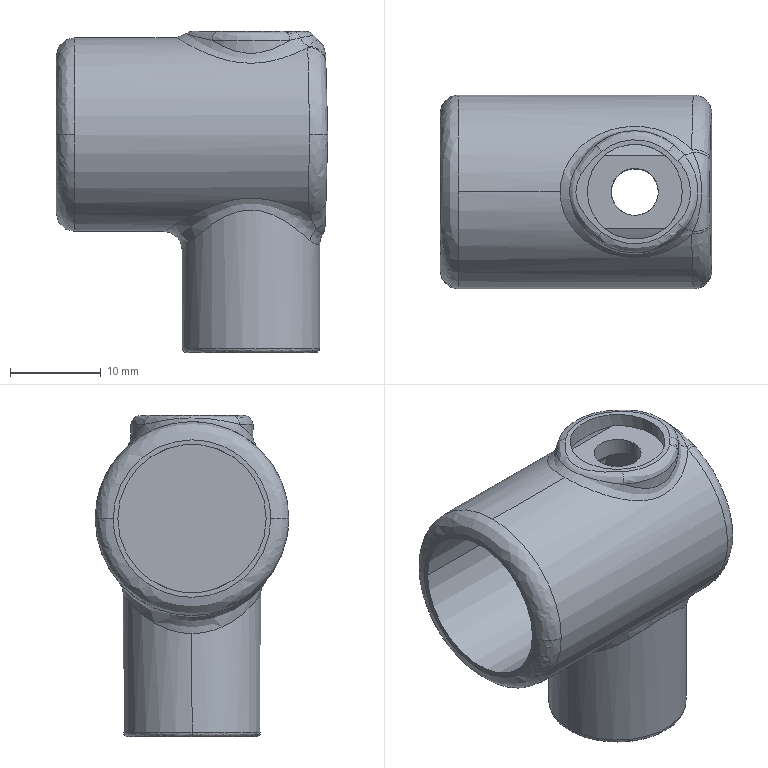Part | SolidWorks | features BaseBody 1 | 1 solid | 47 faces | box 30 x 21.4 x 35.485 mm | volume 7040 mm3 | spline 24 | cylinder 16 | plane 7 | commonest cylinder face diameters 5.2 x4 21.4 x4 10.5 x2 13.5 x2 15.2 x2 16.4 x2